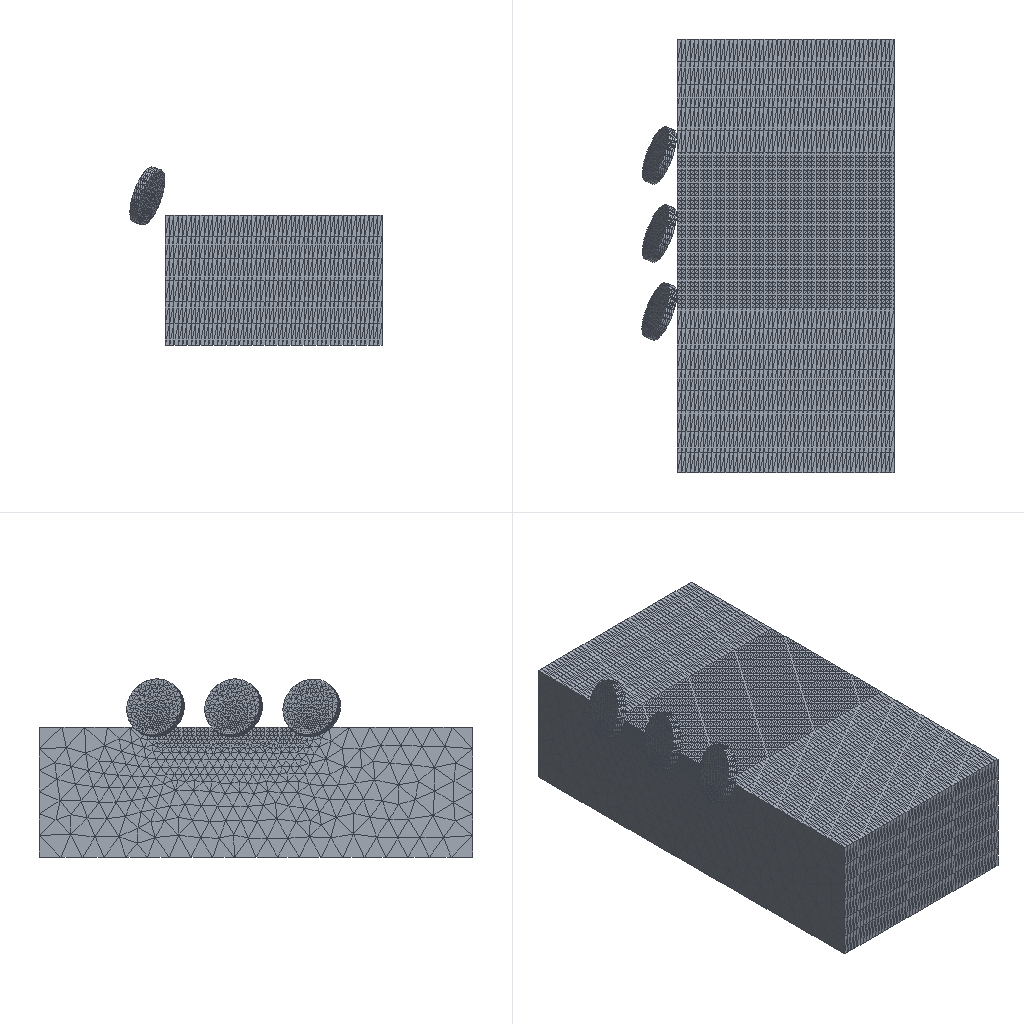Simulation study | abaqus
Set-up summary:
category,name,step,type,value,unit,region
solver,abaqus,,Abaqus/CAE 2024
units,mm-N-s-tonne (MPa),,inferred,E=890000 density=3.54e-09
analysis,Step-1,,dynamic explicit,nlgeom=True; time_period=0.03
mesh,nodes,,,18244
mesh,elements,,,88717
element_type,C3D4T,,,88717
material,tool-PDC,,E,890000
material,tool-PDC,,nu,0.077
material,tool-PDC,,density,3.54e-09
material,tool-PDC,,conductivity,543
material,tool-PDC,,specific_heat,7.9e+08
material,tool-PDC,,behaviors,conductivity; specific heat
material,tool-yingzhihejin,,E,570000
material,tool-yingzhihejin,,nu,0.22
material,tool-yingzhihejin,,density,1.5e-08
material,tool-yingzhihejin,,conductivity,110
material,tool-yingzhihejin,,specific_heat,2.03e+08
material,tool-yingzhihejin,,behaviors,conductivity; specific heat
material,work,,E,40000
material,work,,nu,0.25
material,work,,density,2.65e-09
material,work,,conductivity,3.5
material,work,,specific_heat,7.9e+08
material,work,,behaviors,plastic; conductivity; damage initiation; damage evolution; drucker prager; drucker prager hardening; specific heat
section,tool-PDC,,solid section,,,Set-9
section,tool-PDC,,solid section,,,Set-1
section,work,,solid section,,,Set-15
load,Predefined,initial,initial condition temperature,[n=3]
load,workT,initial,initial condition temperature
bc,BC-1,initial,encastre,[dofs=ENCASTRE],,Set-4
bc,BC-2,Step-1,velocity,"2000 [dofs=rx,ry,rz,x,y,z n=6]",,Set-1
contact,Int-1,Step-1,contact pair,interaction=IntProp-1; friction=0.3; behavior=hard,,tool.toolsurf / work_chipchipaaaaa_CNS_
contact,Int-2,Step-1,contact pair,interaction=IntProp-1; friction=0.3; behavior=hard,,tool_1.toolsurf / work_chipchipaaaaa_CNS_
contact,Int-4,Step-1,contact pair,interaction=IntProp-1; friction=0.3; behavior=hard,,tool_2.tool2surf / work_chipchipaaaaa_CNS_
contact,Int-3,Step-1,general contact,interaction=IntProp-1; friction=0.3; behavior=hard
constraint,rigid body,,,1
Abaqus input file, long lists of numbers shortened:
*Heading
** Job name: deck Model name: Model-1
** Generated by: Abaqus/CAE 2024
*Preprint, echo=NO, model=NO, history=NO, contact=NO
**
** PARTS
**
*Part, name=tool
*Node
      1,           2.,  -4.783,  -4.72
      2,           2.,   4.783,  -4.72
** (1230 more lines like these left out)
*Element, type=C3D4T
   1,  678,  679,  680,  681
   2,  678,  682,  683,  684
** (5239 more lines like these left out)
*Nset, nset=Set-9, generate
    1,  1232,     1
*Elset, elset=Set-9, generate
    1,  5241,     1
*Nset, nset=T-toolTtool
    1,    2,    3,    4,    5,    6,    7,    8,    9,   10,   11,   12,   13,   14,   15,   16
   17,   18,   19,   20,   21,   22,   23,   24,   25,   26,   29,   30,   31,   32,   33,   34
** (75 more lines like these left out)
*Elset, elset=toolRigid, generate
    1,  5241,     1
*Nset, nset=wendu-tool, generate
    1,  1232,     1
*Elset, elset=_toolsurf_S1, internal
  326,  417,  444,  448,  770,  979, 1030, 1118, 1165, 1287, 1396, 1493, 1583, 1616, 1620, 1706
 1792, 1994, 1996, 2158, 2198, 2253, 2411, 2521, 2528, 2612, 2618, 2633, 2812, 2940, 2969, 3002
** (3 more lines like these left out)
*Elset, elset=_toolsurf_S2, internal
  329,  444,  979, 1031, 1242, 1497, 1754, 1996, 2025, 2118, 2158, 2198, 2233, 2236, 2272, 2829
 2949, 3064, 3136, 3161, 3204, 3228, 3405, 3450, 3461, 3476, 3482, 3538, 3575, 3582, 3599, 3640
** (3 more lines like these left out)
*Elset, elset=_toolsurf_S3, internal
   21,   72,  105,  109,  112,  113,  207,  221,  251,  272,  275,  279,  282,  286,  287,  328
  329,  349,  354,  358,  364,  390,  400,  418,  419,  427,  430,  436,  445,  446,  495,  503
** (68 more lines like these left out)
*Elset, elset=_toolsurf_S4, internal
   40,  384,  389,  525,  659,  669,  760,  882,  978, 1037, 1224, 1279, 1384, 1385, 1497, 1558
 1659, 1704, 1778, 1789, 1848, 1935, 2062, 2071, 2168, 2200, 2261, 2324, 2348, 2412, 2477, 2501
** (4 more lines like these left out)
*Surface, type=ELEMENT, name=toolsurf
_toolsurf_S1, S1
_toolsurf_S2, S2
_toolsurf_S4, S4
_toolsurf_S3, S3
** Section: Section-2
*Solid Section, elset=Set-9, material=tool-PDC
,
*End Part
**
*Part, name=tool_2
*Node
      1,           2.,  -4.783,  -4.72
      2,           2.,   4.783,  -4.72
** (1232 more lines like these left out)
*Element, type=C3D4T
   1,  678,  679,  680,  681
   2,  678,  682,  683,  679
** (5258 more lines like these left out)
*Nset, nset=Set-1, generate
    1,  1234,     1
*Elset, elset=Set-1, generate
    1,  5260,     1
*Nset, nset=tool2-T, generate
    1,  1234,     1
*Elset, elset=tool2rigid, generate
    1,  5260,     1
*Elset, elset=_tool2surf_S1, internal
  326,  417,  470,  473,  498,  770,  997, 1002, 1142, 1315, 1348, 1425, 1493, 1616, 1618, 1652
 1766, 1789, 1993, 2054, 2216, 2253, 2314, 2431, 2477, 2521, 2528, 2540, 2611, 2617, 2638, 2812
** (3 more lines like these left out)
*Elset, elset=_tool2surf_S2, internal
  329,  470,  499,  677, 1002, 1242, 1348, 1497, 1682, 1751, 1923, 1993, 2022, 2216, 2232, 2253
 2268, 2646, 2726, 2730, 2829, 2949, 3064, 3161, 3204, 3228, 3236, 3237, 3252, 3328, 3351, 3451
** (3 more lines like these left out)
*Elset, elset=_tool2surf_S3, internal
   21,   72,   92,  112,  113,  133,  137,  207,  237,  253,  272,  329,  358,  364,  374,  400
  418,  419,  427,  445,  449,  455,  471,  494,  503,  504,  522,  544,  560,  575,  578,  585
** (68 more lines like these left out)
*Elset, elset=_tool2surf_S4, internal
  330,  464,  649,  678,  966,  972, 1001, 1019, 1037, 1117, 1245, 1254, 1385, 1497, 1586, 1658
 1659, 1702, 1706, 1786, 1795, 1845, 1932, 2002, 2059, 2068, 2165, 2166, 2229, 2257, 2261, 2345
** (5 more lines like these left out)
*Surface, type=ELEMENT, name=tool2surf
_tool2surf_S1, S1
_tool2surf_S2, S2
_tool2surf_S4, S4
_tool2surf_S3, S3
** Section: tool2
*Solid Section, elset=Set-1, material=tool-PDC
,
*End Part
**
*Part, name=work
*Node
      1,          50.,  -26.243,          28.
      2,          50.,         -62.,          28.
** (14542 more lines like these left out)
*Element, type=C3D4T
    1,  4972,  4973,  4974,  4975
    2,  4972,  4976,  4977,  4978
** (72973 more lines like these left out)
*Nset, nset=Set-15, generate
     1,  14544,      1
*Elset, elset=Set-15, generate
     1,  72975,      1
*Nset, nset=workwenduchang, generate
     1,  14544,      1
*Nset, nset=chipchipaaaaa
     1,     2,     3,     8,     9,    14,    15,    16,    17,    18,    19,    20,    21,    22,    23,    24
    25,    26,    27,    28,    29,    30,    31,    32,    33,    34,    35,    36,    37,    38,    39,    40
** (429 more lines like these left out)
** Section: Section-1
*Solid Section, elset=Set-15, material=work
,
*End Part
**
**
** ASSEMBLY
**
*Assembly, name=Assembly
**
*Instance, name=tool, part=tool
-8.613, -22.209, 64.
-8.613, -22.209, 64., -8.736, -21.507, 63.299, 28.212
*End Instance
**
*Instance, name=tool_1, part=tool
-8.613, -4.209, 64.
-8.613, -4.209, 64., -8.862, -3.524, 63.316, 27.991
*End Instance
**
*Instance, name=work, part=work
-3.613, 40.291, 29.28
*End Instance
**
*Instance, name=tool_2, part=tool_2
-8.613, 13.791, 64.
-8.613, 13.791, 64., -8.862, 14.476, 63.316, 27.991
*End Instance
**
*Node
      1,  -8.613,  -4.209,   64.
*Node
      2,  -8.613,  -22.209,   64.
*Nset, nset=Set-1
 1,
*Nset, nset=Set-2
 2,
*Nset, nset=Set-4, instance=work
    5,    6,   11,   12,   65,   66,   67,   68,   69,   70,   71,   72,   73,   74,   75,   76
   77,   78,   79,   80,   81,   82,   83,  234,  235,  236,  237,  238,  239,  240,  241,  242
** (65 more lines like these left out)
*Elset, elset=Set-4, instance=work
    32,   101,   228,   331,   408,   505,  1083,  1289,  1332,  2379,  2517,  2623,  2714,  3193,  3301,  3311
  3410,  3536,  3543,  3819,  5110,  5709,  6245,  6581,  6586,  6587,  6588,  6611,  6665,  6667,  6671,  6679
** (123 more lines like these left out)
*Nset, nset=b_Set-3, instance=tool_1, generate
    1,  1232,     1
*Elset, elset=b_Set-3, instance=tool_1, generate
    1,  5241,     1
*Nset, nset=b_Set-5, instance=tool, generate
    1,  1232,     1
*Nset, nset=b_Set-5, instance=tool_1, generate
    1,  1232,     1
*Elset, elset=b_Set-5, instance=tool, generate
    1,  5241,     1
*Elset, elset=b_Set-5, instance=tool_1, generate
    1,  5241,     1
*Elset, elset=gangtiall, instance=tool, generate
    1,  5241,     1
*Elset, elset=gangtiall, instance=tool_1, generate
    1,  5241,     1
*Elset, elset=three-rigid, instance=tool, generate
    1,  5241,     1
*Elset, elset=three-rigid, instance=tool_1, generate
    1,  5241,     1
*Elset, elset=three-rigid, instance=tool_2, generate
    1,  5260,     1
*Surface, type=NODE, name=work_chipchipaaaaa_CNS_, internal
work.chipchipaaaaa, 1.
** Constraint: Constraint-1
*Rigid Body, ref node=Set-1, elset=three-rigid
*End Assembly
**
** MATERIALS
**
*Material, name=tool-PDC
*Conductivity
543.,
*Density
 3.54e-09,
*Elastic
890000., 0.077
*Specific Heat
 7.9e+08,
*Material, name=tool-yingzhihejin
*Conductivity
110.,
*Density
 1.5e-08,
*Elastic
570000., 0.22
*Specific Heat
 2.03e+08,
*Material, name=work
*Conductivity
 3.5,
*Damage Initiation, criterion=JOHNSON COOK
 0.02,  0.38, -0.46,    0.,    0., 2000.,   20.,    1.
*Damage Evolution, type=DISPLACEMENT
 0.0002,
*Density
 2.65e-09,
*Drucker Prager
39., 0.95,  15.
*Drucker Prager Hardening, type=SHEAR
100.,0.
*Elastic
40000., 0.25
*Specific Heat
 7.9e+08,
**
** INTERACTION PROPERTIES
**
*Surface Interaction, name=IntProp-1
*Friction
 0.3,
*Surface Behavior, pressure-overclosure=HARD
**
** BOUNDARY CONDITIONS
**
** Name: BC-1 Type: Symmetry/Antisymmetry/Encastre
*Boundary
Set-4, ENCASTRE
**
** PREDEFINED FIELDS
**
** Name: Predefined Field-2   Type: Temperature
*Initial Conditions, type=TEMPERATURE
tool.wendu-tool, 25.
** Name: Predefined Field-3   Type: Temperature
*Initial Conditions, type=TEMPERATURE
tool_1.wendu-tool, 25.
** Name: Predefined Field-4   Type: Temperature
*Initial Conditions, type=TEMPERATURE
tool_2.tool2-T, 25.
** Name: workT   Type: Temperature
*Initial Conditions, type=TEMPERATURE
work.workwenduchang, 25.
** ----------------------------------------------------------------
**
** STEP: Step-1
**
*Step, name=Step-1, nlgeom=YES
*Dynamic, Explicit
, 0.03
*Bulk Viscosity
0.06, 1.2
** Mass Scaling: Semi-Automatic
**               Whole Model
*Fixed Mass Scaling, factor=200.
**
** BOUNDARY CONDITIONS
**
** Name: BC-2 Type: Velocity/Angular velocity
*Boundary, type=VELOCITY
Set-1, 1, 1, 2000.
Set-1, 2, 2
Set-1, 3, 3
Set-1, 4, 4
Set-1, 5, 5
Set-1, 6, 6
**
** INTERACTIONS
**
** Interaction: Int-1
*Contact Pair, interaction=IntProp-1, mechanical constraint=KINEMATIC, cpset=Int-1
tool.toolsurf, work_chipchipaaaaa_CNS_
** Interaction: Int-2
*Contact Pair, interaction=IntProp-1, mechanical constraint=KINEMATIC, cpset=Int-2
tool_1.toolsurf, work_chipchipaaaaa_CNS_
** Interaction: Int-4
*Contact Pair, interaction=IntProp-1, mechanical constraint=KINEMATIC, cpset=Int-4
tool_2.tool2surf, work_chipchipaaaaa_CNS_
** Interaction: Int-3
*Contact, op=NEW
*Contact Inclusions, ALL EXTERIOR
*Contact Property Assignment
 ,  , IntProp-1
**
** OUTPUT REQUESTS
**
*Restart, write, number interval=1, time marks=NO
**
** FIELD OUTPUT: F-Output-1
**
*Output, field, number interval=200
*Node Output
RT, U
*Element Output, directions=YES
MISES, PEEQ, STATUS, TEMP
*Output, history, frequency=0
*End Step
Results summary:
result,odb.job_status,,,JOB_STATUS_COMPLETED_SUCCESSFULLY,"consistent, unstated (Abaqus has no unit system)"
result,steps[0].procedure,Step-1,,"*DYNAMIC, EXPLICIT","consistent, unstated (Abaqus has no unit system)"
result,steps[0].time_period,Step-1,,0.03,"consistent, unstated (Abaqus has no unit system)"
result,steps[0].n_frames,Step-1,,201,"consistent, unstated (Abaqus has no unit system)"
result,steps[0].last_frame.id,Step-1,,86082,"consistent, unstated (Abaqus has no unit system)"
result,steps[0].last_frame.value,Step-1,,0.03,"consistent, unstated (Abaqus has no unit system)"
result,steps[0].last_frame.description,Step-1,,Increment     86082: Step Time =   3.0000E-02,"consistent, unstated (Abaqus has no unit system)"
result,steps[0].completed,Step-1,,True,"consistent, unstated (Abaqus has no unit system)"
result,steps[0].max_U_magnitude,Step-1,,1111.16,"consistent, unstated (Abaqus has no unit system)"
result,steps[0].max_S_mises,Step-1,,567.469,"consistent, unstated (Abaqus has no unit system)"
result,steps[0].diagnostic.n_increments,Step-1,,201,"consistent, unstated (Abaqus has no unit system)"